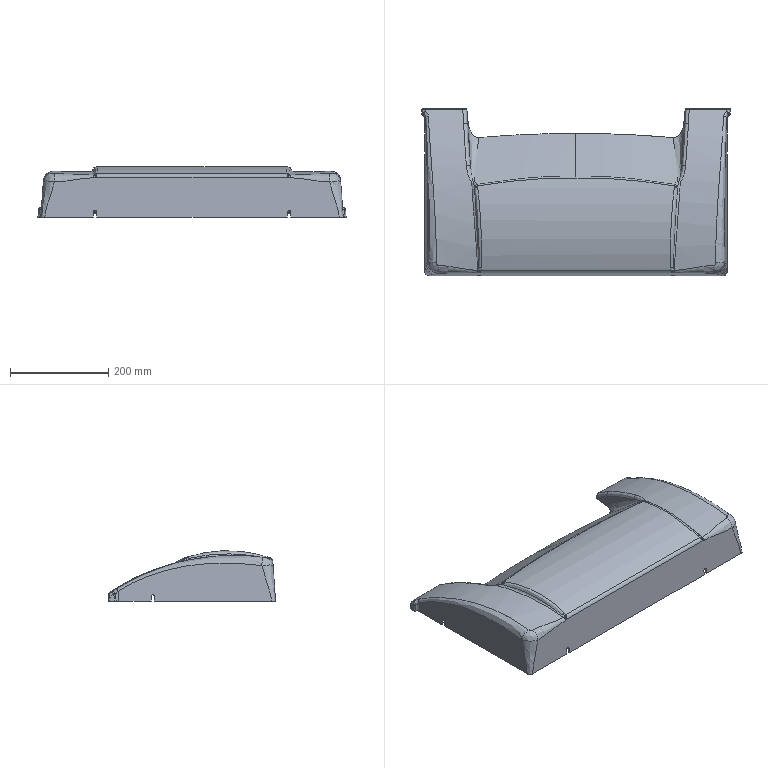Part | STEP file | MOTOR COVER | 1 solid | 258 faces | box 627.004 x 340 x 102.717 mm | volume 823151 mm3 | spline 137 | cylinder 69 | plane 47 | sphere 4 | torus 1 | commonest cylinder face diameters 1 x18 6 x14 7.041 x4 4.009 x3 0.6 x2 0.997 x2